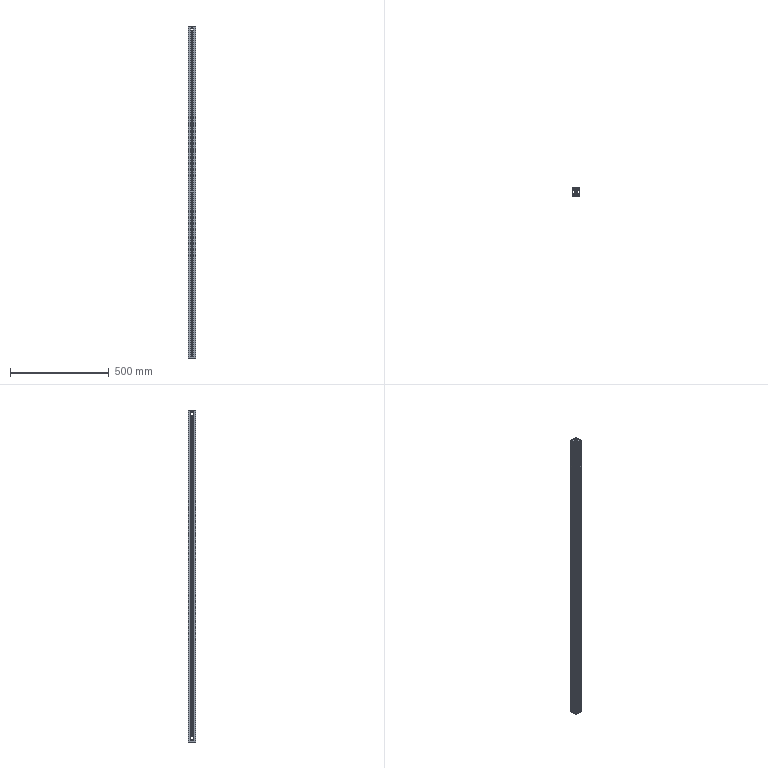Part | SolidWorks | features BaseBody 1, HoleWzd 1, MoveFace 1 | 1 solid | 345 faces | box 40 x 40 x 1682 mm | volume 894323 mm3 | plane 250 | cylinder 95 | commonest cylinder face diameters 0.6 x24 10 x24 2 x16 6.8 x15 19 x12 3 x4